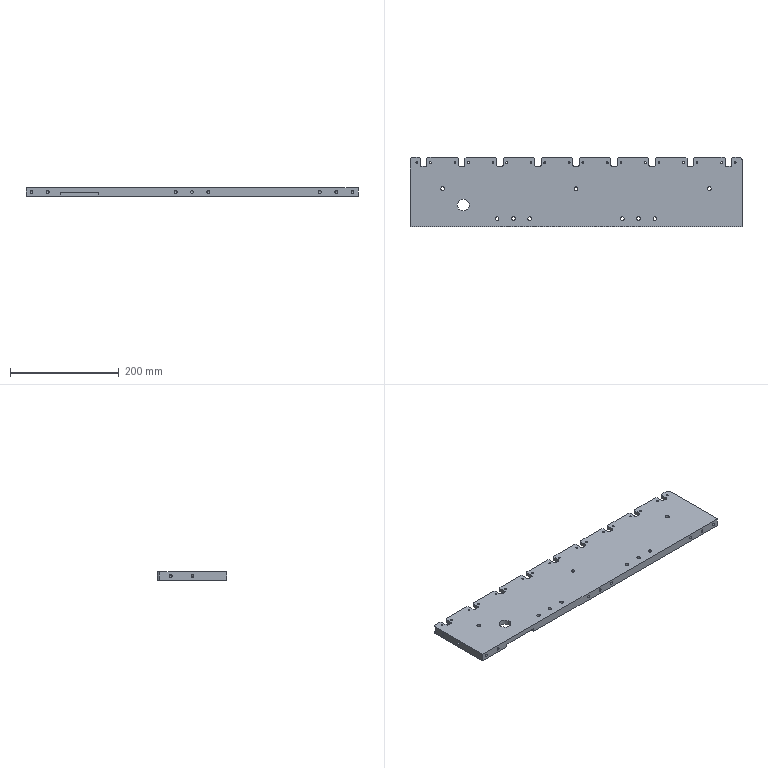Part | NX | 1 solid | 199 faces | box 610 x 128 x 15 mm | volume 1027284 mm3 | plane 107 | cylinder 82 | cone 10 | commonest cylinder face diameters 6 x36 3.3 x18 5 x10 6.6 x6 11 x6 6.8 x3